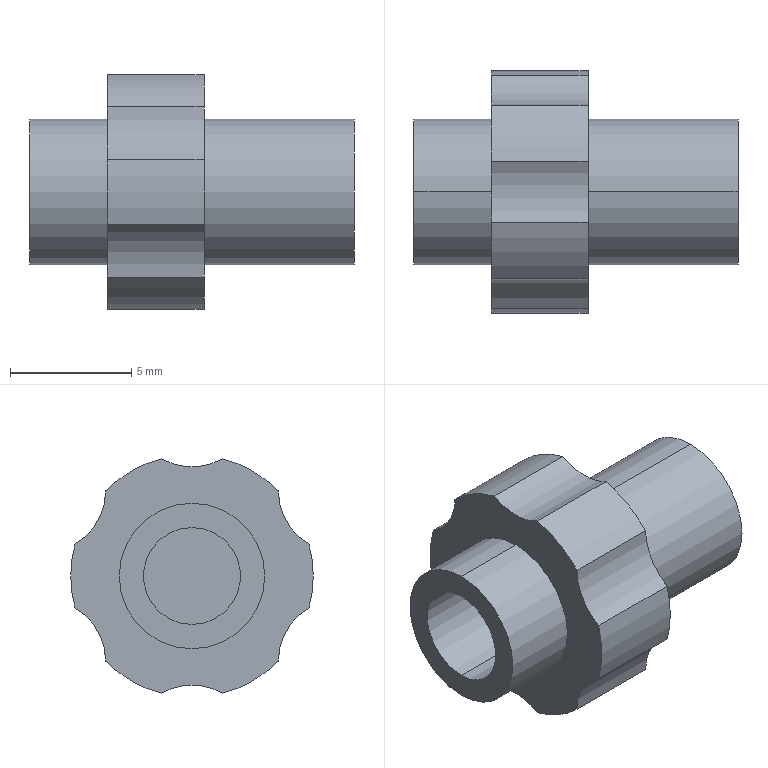Part | STEP file | Dual Brake Lever Cable Adjuster | 1 solid | 24 faces | box 13.365 x 10 x 9.679 mm | volume 483.226 mm3 | cylinder 19 | plane 5 | commonest cylinder face diameters 5 x7 10 x6 6 x4 4 x2